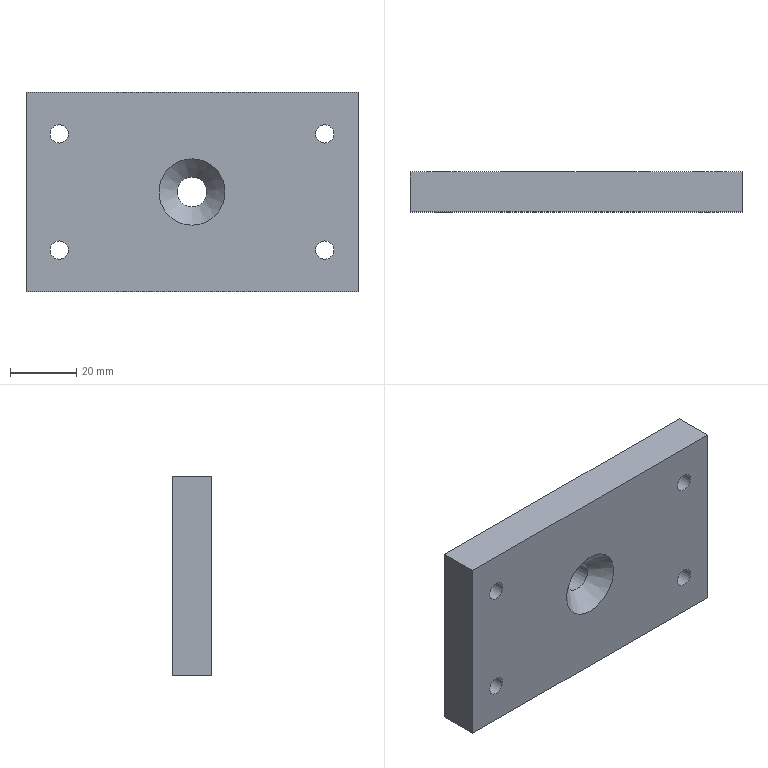Part | STEP file | 1 solid | 33 faces | box 100 x 12 x 60 mm | volume 66467 mm3 | plane 15 | cylinder 13 | cone 5 | commonest cylinder face diameters 5 x4 5.5 x4 10 x4 9 x1